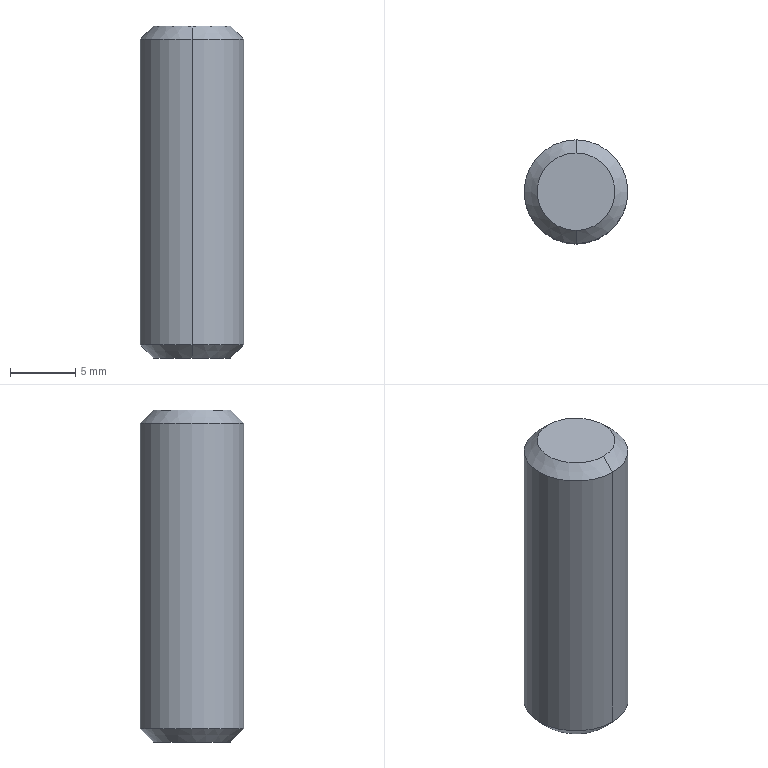Part | NX | features BREP 1 | 1 solid | 8 faces | box 7.938 x 7.938 x 25.4 mm | volume 1234 mm3 | cone 4 | plane 2 | cylinder 2 | commonest cylinder face diameters 7.938 x2
STEP:
#1=CARTESIAN_POINT('',(0.,2.969,0.));
#2=VERTEX_POINT('',#1);
#3=CARTESIAN_POINT('',(0.,-2.969,0.));
#4=VERTEX_POINT('',#3);
#5=CARTESIAN_POINT('',(0.,0.,0.));
#6=DIRECTION('',(0.,0.,-1.));
#7=DIRECTION('',(0.,1.,0.));
#8=AXIS2_PLACEMENT_3D('',#5,#6,#7);
#9=CIRCLE('',#8,2.969);
#10=EDGE_CURVE('',#2,#4,#9,.T.);
#11=ORIENTED_EDGE('',*,*,#10,.F.);
#12=CARTESIAN_POINT('',(0.,0.,0.));
#13=DIRECTION('',(0.,0.,-1.));
#14=DIRECTION('',(0.,-1.,0.));
#15=AXIS2_PLACEMENT_3D('',#12,#13,#14);
#16=CIRCLE('',#15,2.969);
#17=EDGE_CURVE('',#4,#2,#16,.T.);
#18=ORIENTED_EDGE('',*,*,#17,.F.);
#19=EDGE_LOOP('',(#11,#18));
#20=FACE_BOUND('',#19,.T.);
#21=CARTESIAN_POINT('',(0.,0.,0.));
#22=DIRECTION('',(0.,0.,-1.));
#23=DIRECTION('',(0.,-1.,0.));
#24=AXIS2_PLACEMENT_3D('',#21,#22,#23);
#25=PLANE('',#24);
#26=ADVANCED_FACE('',(#20),#25,.F.);
#27=CARTESIAN_POINT('',(0.,3.969,-1.));
#28=VERTEX_POINT('',#27);
#29=CARTESIAN_POINT('',(0.,2.969,0.));
#30=DIRECTION('',(0.,0.7071,-0.7071));
#31=VECTOR('',#30,1000.);
#32=LINE('',#29,#31);
#33=EDGE_CURVE('',#28,#2,#32,.F.);
#34=ORIENTED_EDGE('',*,*,#33,.F.);
#35=CARTESIAN_POINT('',(0.,-3.969,-1.));
#36=VERTEX_POINT('',#35);
#37=CARTESIAN_POINT('',(0.,0.,-1.));
#38=DIRECTION('',(0.,0.,-1.));
#39=DIRECTION('',(0.,-1.,0.));
#40=AXIS2_PLACEMENT_3D('',#37,#38,#39);
#41=CIRCLE('',#40,3.969);
#42=EDGE_CURVE('',#36,#28,#41,.T.);
#43=ORIENTED_EDGE('',*,*,#42,.F.);
#44=CARTESIAN_POINT('',(0.,-2.969,0.));
#45=DIRECTION('',(0.,-0.7071,-0.7071));
#46=VECTOR('',#45,1000.);
#47=LINE('',#44,#46);
#48=EDGE_CURVE('',#36,#4,#47,.F.);
#49=ORIENTED_EDGE('',*,*,#48,.T.);
#50=ORIENTED_EDGE('',*,*,#17,.T.);
#51=EDGE_LOOP('',(#34,#43,#49,#50));
#52=FACE_BOUND('',#51,.T.);
#53=CARTESIAN_POINT('',(0.,0.,-0.5));
#54=DIRECTION('',(0.,0.,-1.));
#55=DIRECTION('',(0.,-1.,0.));
#56=AXIS2_PLACEMENT_3D('',#53,#54,#55);
#57=CONICAL_SURFACE('',#56,3.469,0.7854);
#58=ADVANCED_FACE('',(#52),#57,.T.);
#59=ORIENTED_EDGE('',*,*,#48,.F.);
#60=CARTESIAN_POINT('',(0.,0.,-1.));
#61=DIRECTION('',(0.,0.,-1.));
#62=DIRECTION('',(0.,1.,0.));
#63=AXIS2_PLACEMENT_3D('',#60,#61,#62);
#64=CIRCLE('',#63,3.969);
#65=EDGE_CURVE('',#28,#36,#64,.T.);
#66=ORIENTED_EDGE('',*,*,#65,.F.);
#67=ORIENTED_EDGE('',*,*,#33,.T.);
#68=ORIENTED_EDGE('',*,*,#10,.T.);
#69=EDGE_LOOP('',(#59,#66,#67,#68));
#70=FACE_BOUND('',#69,.T.);
#71=CARTESIAN_POINT('',(0.,0.,-0.5));
#72=DIRECTION('',(0.,0.,-1.));
#73=DIRECTION('',(0.,-1.,0.));
#74=AXIS2_PLACEMENT_3D('',#71,#72,#73);
#75=CONICAL_SURFACE('',#74,3.469,0.7854);
#76=ADVANCED_FACE('',(#70),#75,.T.);
#77=CARTESIAN_POINT('',(0.,-3.969,-24.4));
#78=VERTEX_POINT('',#77);
#79=CARTESIAN_POINT('',(0.,-3.969,-1.));
#80=DIRECTION('',(0.,0.,-1.));
#81=VECTOR('',#80,1000.);
#82=LINE('',#79,#81);
#83=EDGE_CURVE('',#36,#78,#82,.T.);
#84=ORIENTED_EDGE('',*,*,#83,.T.);
#85=CARTESIAN_POINT('',(0.,3.969,-24.4));
#86=VERTEX_POINT('',#85);
#87=CARTESIAN_POINT('',(0.,0.,-24.4));
#88=DIRECTION('',(0.,0.,-1.));
#89=DIRECTION('',(0.,1.,0.));
#90=AXIS2_PLACEMENT_3D('',#87,#88,#89);
#91=CIRCLE('',#90,3.969);
#92=EDGE_CURVE('',#86,#78,#91,.T.);
#93=ORIENTED_EDGE('',*,*,#92,.F.);
#94=CARTESIAN_POINT('',(0.,3.969,-1.));
#95=DIRECTION('',(0.,0.,-1.));
#96=VECTOR('',#95,1000.);
#97=LINE('',#94,#96);
#98=EDGE_CURVE('',#28,#86,#97,.T.);
#99=ORIENTED_EDGE('',*,*,#98,.F.);
#100=ORIENTED_EDGE('',*,*,#65,.T.);
#101=EDGE_LOOP('',(#84,#93,#99,#100));
#102=FACE_BOUND('',#101,.T.);
#103=CARTESIAN_POINT('',(0.,0.,0.));
#104=DIRECTION('',(0.,0.,-1.));
#105=DIRECTION('',(0.,-1.,0.));
#106=AXIS2_PLACEMENT_3D('',#103,#104,#105);
#107=CYLINDRICAL_SURFACE('',#106,3.969);
#108=ADVANCED_FACE('',(#102),#107,.T.);
#109=ORIENTED_EDGE('',*,*,#98,.T.);
#110=CARTESIAN_POINT('',(0.,0.,-24.4));
#111=DIRECTION('',(0.,0.,-1.));
#112=DIRECTION('',(0.,-1.,0.));
#113=AXIS2_PLACEMENT_3D('',#110,#111,#112);
#114=CIRCLE('',#113,3.969);
#115=EDGE_CURVE('',#78,#86,#114,.T.);
#116=ORIENTED_EDGE('',*,*,#115,.F.);
#117=ORIENTED_EDGE('',*,*,#83,.F.);
#118=ORIENTED_EDGE('',*,*,#42,.T.);
#119=EDGE_LOOP('',(#109,#116,#117,#118));
#120=FACE_BOUND('',#119,.T.);
#121=CARTESIAN_POINT('',(0.,0.,0.));
#122=DIRECTION('',(0.,0.,-1.));
#123=DIRECTION('',(0.,-1.,0.));
#124=AXIS2_PLACEMENT_3D('',#121,#122,#123);
#125=CYLINDRICAL_SURFACE('',#124,3.969);
#126=ADVANCED_FACE('',(#120),#125,.T.);
#127=CARTESIAN_POINT('',(0.,-2.969,-25.4));
#128=VERTEX_POINT('',#127);
#129=CARTESIAN_POINT('',(0.,-2.969,-25.4));
#130=DIRECTION('',(0.,-0.7071,0.7071));
#131=VECTOR('',#130,1000.);
#132=LINE('',#129,#131);
#133=EDGE_CURVE('',#128,#78,#132,.T.);
#134=ORIENTED_EDGE('',*,*,#133,.T.);
#135=ORIENTED_EDGE('',*,*,#115,.T.);
#136=CARTESIAN_POINT('',(0.,2.969,-25.4));
#137=VERTEX_POINT('',#136);
#138=CARTESIAN_POINT('',(0.,2.969,-25.4));
#139=DIRECTION('',(0.,0.7071,0.7071));
#140=VECTOR('',#139,1000.);
#141=LINE('',#138,#140);
#142=EDGE_CURVE('',#137,#86,#141,.T.);
#143=ORIENTED_EDGE('',*,*,#142,.F.);
#144=CARTESIAN_POINT('',(0.,0.,-25.4));
#145=DIRECTION('',(0.,0.,-1.));
#146=DIRECTION('',(0.,-1.,0.));
#147=AXIS2_PLACEMENT_3D('',#144,#145,#146);
#148=CIRCLE('',#147,2.969);
#149=EDGE_CURVE('',#128,#137,#148,.T.);
#150=ORIENTED_EDGE('',*,*,#149,.F.);
#151=EDGE_LOOP('',(#134,#135,#143,#150));
#152=FACE_BOUND('',#151,.T.);
#153=CARTESIAN_POINT('',(0.,0.,-24.9));
#154=DIRECTION('',(0.,0.,1.));
#155=DIRECTION('',(0.,1.,0.));
#156=AXIS2_PLACEMENT_3D('',#153,#154,#155);
#157=CONICAL_SURFACE('',#156,3.469,0.7854);
#158=ADVANCED_FACE('',(#152),#157,.T.);
#159=CARTESIAN_POINT('',(0.,0.,-25.4));
#160=DIRECTION('',(0.,0.,-1.));
#161=DIRECTION('',(0.,1.,0.));
#162=AXIS2_PLACEMENT_3D('',#159,#160,#161);
#163=CIRCLE('',#162,2.969);
#164=EDGE_CURVE('',#137,#128,#163,.T.);
#165=ORIENTED_EDGE('',*,*,#164,.T.);
#166=ORIENTED_EDGE('',*,*,#149,.T.);
#167=EDGE_LOOP('',(#165,#166));
#168=FACE_BOUND('',#167,.T.);
#169=CARTESIAN_POINT('',(0.,0.,-25.4));
#170=DIRECTION('',(0.,0.,-1.));
#171=DIRECTION('',(0.,-1.,0.));
#172=AXIS2_PLACEMENT_3D('',#169,#170,#171);
#173=PLANE('',#172);
#174=ADVANCED_FACE('',(#168),#173,.T.);
#175=ORIENTED_EDGE('',*,*,#142,.T.);
#176=ORIENTED_EDGE('',*,*,#92,.T.);
#177=ORIENTED_EDGE('',*,*,#133,.F.);
#178=ORIENTED_EDGE('',*,*,#164,.F.);
#179=EDGE_LOOP('',(#175,#176,#177,#178));
#180=FACE_BOUND('',#179,.T.);
#181=CARTESIAN_POINT('',(0.,0.,-24.9));
#182=DIRECTION('',(0.,0.,1.));
#183=DIRECTION('',(0.,1.,0.));
#184=AXIS2_PLACEMENT_3D('',#181,#182,#183);
#185=CONICAL_SURFACE('',#184,3.469,0.7854);
#186=ADVANCED_FACE('',(#180),#185,.T.);
#187=CLOSED_SHELL('',(#26,#58,#76,#108,#126,#158,#174,#186));
#188=MANIFOLD_SOLID_BREP('',#187);
#189=(LENGTH_UNIT()NAMED_UNIT(*)SI_UNIT(.MILLI.,.METRE.));
#190=UNCERTAINTY_MEASURE_WITH_UNIT(LENGTH_MEASURE(0.00001),#189,'','');
#191=(NAMED_UNIT(*)PLANE_ANGLE_UNIT()SI_UNIT($,.RADIAN.));
#192=(NAMED_UNIT(*)SI_UNIT($,.STERADIAN.)SOLID_ANGLE_UNIT());
#193=(GEOMETRIC_REPRESENTATION_CONTEXT(3)GLOBAL_UNCERTAINTY_ASSIGNED_CONTEXT((#190))GLOBAL_UNIT_ASSIGNED_CONTEXT((#189,#191,#192))REPRESENTATION_CONTEXT('',''));
#194=ADVANCED_BREP_SHAPE_REPRESENTATION('',(#188),#193);